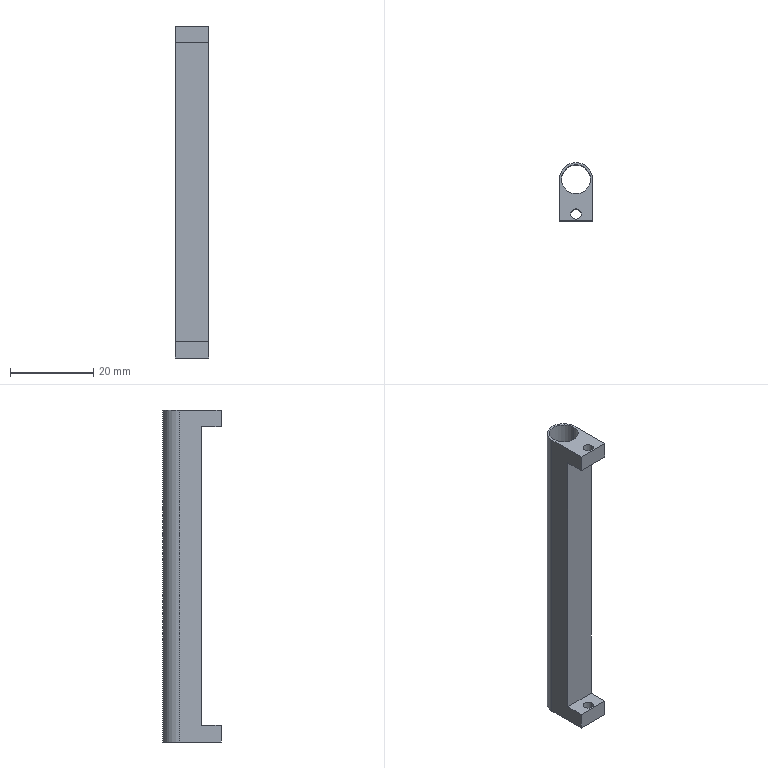Part | SolidWorks | features BaseBody 1 | 1 solid | 17 faces | box 8 x 14 x 80 mm | volume 2633 mm3 | plane 9 | cylinder 8 | commonest cylinder face diameters 2.5 x4 7 x2 8 x2
STEP:
#1=CARTESIAN_POINT('',(-1.25,-5.382,0.));
#2=VERTEX_POINT('',#1);
#3=CARTESIAN_POINT('',(1.25,-5.382,0.));
#4=VERTEX_POINT('',#3);
#5=CARTESIAN_POINT('',(0.,-5.382,0.));
#6=DIRECTION('',(0.,0.,1.));
#7=DIRECTION('',(1.,0.,0.));
#8=AXIS2_PLACEMENT_3D('',#5,#6,#7);
#9=CIRCLE('',#8,1.25);
#10=EDGE_CURVE('',#2,#4,#9,.T.);
#11=ORIENTED_EDGE('',*,*,#10,.F.);
#12=CARTESIAN_POINT('',(-1.25,-5.382,4.));
#13=VERTEX_POINT('',#12);
#14=CARTESIAN_POINT('',(-1.25,-5.382,0.));
#15=DIRECTION('',(0.,0.,1.));
#16=VECTOR('',#15,1000.);
#17=LINE('',#14,#16);
#18=EDGE_CURVE('',#2,#13,#17,.T.);
#19=ORIENTED_EDGE('',*,*,#18,.T.);
#20=CARTESIAN_POINT('',(1.25,-5.382,4.));
#21=VERTEX_POINT('',#20);
#22=CARTESIAN_POINT('',(0.,-5.382,4.));
#23=DIRECTION('',(0.,0.,1.));
#24=DIRECTION('',(1.,0.,0.));
#25=AXIS2_PLACEMENT_3D('',#22,#23,#24);
#26=CIRCLE('',#25,1.25);
#27=EDGE_CURVE('',#13,#21,#26,.T.);
#28=ORIENTED_EDGE('',*,*,#27,.T.);
#29=CARTESIAN_POINT('',(1.25,-5.382,0.));
#30=DIRECTION('',(0.,0.,1.));
#31=VECTOR('',#30,1000.);
#32=LINE('',#29,#31);
#33=EDGE_CURVE('',#4,#21,#32,.T.);
#34=ORIENTED_EDGE('',*,*,#33,.F.);
#35=EDGE_LOOP('',(#11,#19,#28,#34));
#36=FACE_OUTER_BOUND('',#35,.T.);
#37=CARTESIAN_POINT('',(0.,-5.382,0.));
#38=DIRECTION('',(0.,0.,1.));
#39=DIRECTION('',(1.,0.,0.));
#40=AXIS2_PLACEMENT_3D('',#37,#38,#39);
#41=CYLINDRICAL_SURFACE('',#40,1.25);
#42=ADVANCED_FACE('',(#36),#41,.F.);
#43=CARTESIAN_POINT('',(-1.25,-5.382,76.));
#44=VERTEX_POINT('',#43);
#45=CARTESIAN_POINT('',(1.25,-5.382,76.));
#46=VERTEX_POINT('',#45);
#47=CARTESIAN_POINT('',(0.,-5.382,76.));
#48=DIRECTION('',(0.,0.,1.));
#49=DIRECTION('',(1.,0.,0.));
#50=AXIS2_PLACEMENT_3D('',#47,#48,#49);
#51=CIRCLE('',#50,1.25);
#52=EDGE_CURVE('',#44,#46,#51,.T.);
#53=ORIENTED_EDGE('',*,*,#52,.F.);
#54=CARTESIAN_POINT('',(-1.25,-5.382,80.));
#55=VERTEX_POINT('',#54);
#56=CARTESIAN_POINT('',(-1.25,-5.382,0.));
#57=DIRECTION('',(0.,0.,1.));
#58=VECTOR('',#57,1000.);
#59=LINE('',#56,#58);
#60=EDGE_CURVE('',#44,#55,#59,.T.);
#61=ORIENTED_EDGE('',*,*,#60,.T.);
#62=CARTESIAN_POINT('',(1.25,-5.382,80.));
#63=VERTEX_POINT('',#62);
#64=CARTESIAN_POINT('',(0.,-5.382,80.));
#65=DIRECTION('',(0.,0.,1.));
#66=DIRECTION('',(1.,0.,0.));
#67=AXIS2_PLACEMENT_3D('',#64,#65,#66);
#68=CIRCLE('',#67,1.25);
#69=EDGE_CURVE('',#55,#63,#68,.T.);
#70=ORIENTED_EDGE('',*,*,#69,.T.);
#71=CARTESIAN_POINT('',(1.25,-5.382,0.));
#72=DIRECTION('',(0.,0.,1.));
#73=VECTOR('',#72,1000.);
#74=LINE('',#71,#73);
#75=EDGE_CURVE('',#46,#63,#74,.T.);
#76=ORIENTED_EDGE('',*,*,#75,.F.);
#77=EDGE_LOOP('',(#53,#61,#70,#76));
#78=FACE_OUTER_BOUND('',#77,.T.);
#79=CARTESIAN_POINT('',(0.,-5.382,0.));
#80=DIRECTION('',(0.,0.,1.));
#81=DIRECTION('',(1.,0.,0.));
#82=AXIS2_PLACEMENT_3D('',#79,#80,#81);
#83=CYLINDRICAL_SURFACE('',#82,1.25);
#84=ADVANCED_FACE('',(#78),#83,.F.);
#85=CARTESIAN_POINT('',(3.5,3.,80.));
#86=VERTEX_POINT('',#85);
#87=CARTESIAN_POINT('',(-3.5,3.,80.));
#88=VERTEX_POINT('',#87);
#89=CARTESIAN_POINT('',(0.,3.,80.));
#90=DIRECTION('',(0.,0.,-1.));
#91=DIRECTION('',(-1.,0.,0.));
#92=AXIS2_PLACEMENT_3D('',#89,#90,#91);
#93=CIRCLE('',#92,3.5);
#94=EDGE_CURVE('',#86,#88,#93,.T.);
#95=ORIENTED_EDGE('',*,*,#94,.F.);
#96=CARTESIAN_POINT('',(3.5,3.,0.));
#97=VERTEX_POINT('',#96);
#98=CARTESIAN_POINT('',(3.5,3.,80.));
#99=DIRECTION('',(0.,0.,-1.));
#100=VECTOR('',#99,1000.);
#101=LINE('',#98,#100);
#102=EDGE_CURVE('',#86,#97,#101,.T.);
#103=ORIENTED_EDGE('',*,*,#102,.T.);
#104=CARTESIAN_POINT('',(-3.5,3.,0.));
#105=VERTEX_POINT('',#104);
#106=CARTESIAN_POINT('',(0.,3.,0.));
#107=DIRECTION('',(0.,0.,-1.));
#108=DIRECTION('',(-1.,0.,0.));
#109=AXIS2_PLACEMENT_3D('',#106,#107,#108);
#110=CIRCLE('',#109,3.5);
#111=EDGE_CURVE('',#97,#105,#110,.T.);
#112=ORIENTED_EDGE('',*,*,#111,.T.);
#113=CARTESIAN_POINT('',(-3.5,3.,80.));
#114=DIRECTION('',(0.,0.,-1.));
#115=VECTOR('',#114,1000.);
#116=LINE('',#113,#115);
#117=EDGE_CURVE('',#88,#105,#116,.T.);
#118=ORIENTED_EDGE('',*,*,#117,.F.);
#119=EDGE_LOOP('',(#95,#103,#112,#118));
#120=FACE_OUTER_BOUND('',#119,.T.);
#121=CARTESIAN_POINT('',(0.,3.,80.));
#122=DIRECTION('',(0.,0.,-1.));
#123=DIRECTION('',(-1.,0.,0.));
#124=AXIS2_PLACEMENT_3D('',#121,#122,#123);
#125=CYLINDRICAL_SURFACE('',#124,3.5);
#126=ADVANCED_FACE('',(#120),#125,.F.);
#127=CARTESIAN_POINT('',(4.,-7.,4.));
#128=VERTEX_POINT('',#127);
#129=CARTESIAN_POINT('',(4.,-7.,0.));
#130=VERTEX_POINT('',#129);
#131=CARTESIAN_POINT('',(4.,-7.,80.));
#132=DIRECTION('',(0.,0.,-1.));
#133=VECTOR('',#132,1000.);
#134=LINE('',#131,#133);
#135=EDGE_CURVE('',#128,#130,#134,.T.);
#136=ORIENTED_EDGE('',*,*,#135,.F.);
#137=CARTESIAN_POINT('',(-4.,-7.,4.));
#138=VERTEX_POINT('',#137);
#139=CARTESIAN_POINT('',(-4.,-7.,4.));
#140=DIRECTION('',(1.,0.,0.));
#141=VECTOR('',#140,1000.);
#142=LINE('',#139,#141);
#143=EDGE_CURVE('',#138,#128,#142,.T.);
#144=ORIENTED_EDGE('',*,*,#143,.F.);
#145=CARTESIAN_POINT('',(-4.,-7.,0.));
#146=VERTEX_POINT('',#145);
#147=CARTESIAN_POINT('',(-4.,-7.,80.));
#148=DIRECTION('',(0.,0.,-1.));
#149=VECTOR('',#148,1000.);
#150=LINE('',#147,#149);
#151=EDGE_CURVE('',#138,#146,#150,.T.);
#152=ORIENTED_EDGE('',*,*,#151,.T.);
#153=CARTESIAN_POINT('',(-4.,-7.,0.));
#154=DIRECTION('',(1.,0.,0.));
#155=VECTOR('',#154,1000.);
#156=LINE('',#153,#155);
#157=EDGE_CURVE('',#146,#130,#156,.T.);
#158=ORIENTED_EDGE('',*,*,#157,.T.);
#159=EDGE_LOOP('',(#136,#144,#152,#158));
#160=FACE_OUTER_BOUND('',#159,.T.);
#161=CARTESIAN_POINT('',(-4.,-7.,80.));
#162=DIRECTION('',(0.,1.,0.));
#163=DIRECTION('',(0.,0.,1.));
#164=AXIS2_PLACEMENT_3D('',#161,#162,#163);
#165=PLANE('',#164);
#166=ADVANCED_FACE('',(#160),#165,.F.);
#167=CARTESIAN_POINT('',(-4.,-7.,80.));
#168=VERTEX_POINT('',#167);
#169=CARTESIAN_POINT('',(-4.,-7.,76.));
#170=VERTEX_POINT('',#169);
#171=CARTESIAN_POINT('',(-4.,-7.,80.));
#172=DIRECTION('',(0.,0.,-1.));
#173=VECTOR('',#172,1000.);
#174=LINE('',#171,#173);
#175=EDGE_CURVE('',#168,#170,#174,.T.);
#176=ORIENTED_EDGE('',*,*,#175,.T.);
#177=CARTESIAN_POINT('',(4.,-7.,76.));
#178=VERTEX_POINT('',#177);
#179=CARTESIAN_POINT('',(-4.,-7.,76.));
#180=DIRECTION('',(1.,0.,0.));
#181=VECTOR('',#180,1000.);
#182=LINE('',#179,#181);
#183=EDGE_CURVE('',#170,#178,#182,.T.);
#184=ORIENTED_EDGE('',*,*,#183,.T.);
#185=CARTESIAN_POINT('',(4.,-7.,80.));
#186=VERTEX_POINT('',#185);
#187=CARTESIAN_POINT('',(4.,-7.,80.));
#188=DIRECTION('',(0.,0.,-1.));
#189=VECTOR('',#188,1000.);
#190=LINE('',#187,#189);
#191=EDGE_CURVE('',#186,#178,#190,.T.);
#192=ORIENTED_EDGE('',*,*,#191,.F.);
#193=CARTESIAN_POINT('',(-4.,-7.,80.));
#194=DIRECTION('',(1.,0.,0.));
#195=VECTOR('',#194,1000.);
#196=LINE('',#193,#195);
#197=EDGE_CURVE('',#168,#186,#196,.T.);
#198=ORIENTED_EDGE('',*,*,#197,.F.);
#199=EDGE_LOOP('',(#176,#184,#192,#198));
#200=FACE_OUTER_BOUND('',#199,.T.);
#201=CARTESIAN_POINT('',(-4.,-7.,80.));
#202=DIRECTION('',(0.,1.,0.));
#203=DIRECTION('',(0.,0.,1.));
#204=AXIS2_PLACEMENT_3D('',#201,#202,#203);
#205=PLANE('',#204);
#206=ADVANCED_FACE('',(#200),#205,.F.);
#207=CARTESIAN_POINT('',(4.,-2.382,4.));
#208=VERTEX_POINT('',#207);
#209=CARTESIAN_POINT('',(4.,-2.382,76.));
#210=VERTEX_POINT('',#209);
#211=CARTESIAN_POINT('',(4.,-2.382,4.));
#212=DIRECTION('',(0.,0.,1.));
#213=VECTOR('',#212,1000.);
#214=LINE('',#211,#213);
#215=EDGE_CURVE('',#208,#210,#214,.T.);
#216=ORIENTED_EDGE('',*,*,#215,.F.);
#217=CARTESIAN_POINT('',(4.,-7.,4.));
#218=DIRECTION('',(0.,1.,0.));
#219=VECTOR('',#218,1000.);
#220=LINE('',#217,#219);
#221=EDGE_CURVE('',#128,#208,#220,.T.);
#222=ORIENTED_EDGE('',*,*,#221,.F.);
#223=ORIENTED_EDGE('',*,*,#135,.T.);
#224=CARTESIAN_POINT('',(4.,3.,0.));
#225=VERTEX_POINT('',#224);
#226=CARTESIAN_POINT('',(4.,7.,0.));
#227=DIRECTION('',(0.,1.,0.));
#228=VECTOR('',#227,1000.);
#229=LINE('',#226,#228);
#230=EDGE_CURVE('',#130,#225,#229,.T.);
#231=ORIENTED_EDGE('',*,*,#230,.T.);
#232=CARTESIAN_POINT('',(4.,3.,80.));
#233=VERTEX_POINT('',#232);
#234=CARTESIAN_POINT('',(4.,3.,80.));
#235=DIRECTION('',(0.,0.,1.));
#236=VECTOR('',#235,1000.);
#237=LINE('',#234,#236);
#238=EDGE_CURVE('',#225,#233,#237,.T.);
#239=ORIENTED_EDGE('',*,*,#238,.T.);
#240=CARTESIAN_POINT('',(4.,7.,80.));
#241=DIRECTION('',(0.,1.,0.));
#242=VECTOR('',#241,1000.);
#243=LINE('',#240,#242);
#244=EDGE_CURVE('',#186,#233,#243,.T.);
#245=ORIENTED_EDGE('',*,*,#244,.F.);
#246=ORIENTED_EDGE('',*,*,#191,.T.);
#247=CARTESIAN_POINT('',(4.,-7.,76.));
#248=DIRECTION('',(0.,-1.,0.));
#249=VECTOR('',#248,1000.);
#250=LINE('',#247,#249);
#251=EDGE_CURVE('',#210,#178,#250,.T.);
#252=ORIENTED_EDGE('',*,*,#251,.F.);
#253=EDGE_LOOP('',(#216,#222,#223,#231,#239,#245,#246,#252));
#254=FACE_OUTER_BOUND('',#253,.T.);
#255=CARTESIAN_POINT('',(4.,7.,80.));
#256=DIRECTION('',(-1.,0.,0.));
#257=DIRECTION('',(0.,0.,1.));
#258=AXIS2_PLACEMENT_3D('',#255,#256,#257);
#259=PLANE('',#258);
#260=ADVANCED_FACE('',(#254),#259,.F.);
#261=ORIENTED_EDGE('',*,*,#151,.F.);
#262=CARTESIAN_POINT('',(-4.,-2.382,4.));
#263=VERTEX_POINT('',#262);
#264=CARTESIAN_POINT('',(-4.,7.,4.));
#265=DIRECTION('',(0.,1.,0.));
#266=VECTOR('',#265,1000.);
#267=LINE('',#264,#266);
#268=EDGE_CURVE('',#138,#263,#267,.T.);
#269=ORIENTED_EDGE('',*,*,#268,.T.);
#270=CARTESIAN_POINT('',(-4.,-2.382,76.));
#271=VERTEX_POINT('',#270);
#272=CARTESIAN_POINT('',(-4.,-2.382,80.));
#273=DIRECTION('',(0.,0.,1.));
#274=VECTOR('',#273,1000.);
#275=LINE('',#272,#274);
#276=EDGE_CURVE('',#263,#271,#275,.T.);
#277=ORIENTED_EDGE('',*,*,#276,.T.);
#278=CARTESIAN_POINT('',(-4.,7.,76.));
#279=DIRECTION('',(0.,-1.,0.));
#280=VECTOR('',#279,1000.);
#281=LINE('',#278,#280);
#282=EDGE_CURVE('',#271,#170,#281,.T.);
#283=ORIENTED_EDGE('',*,*,#282,.T.);
#284=ORIENTED_EDGE('',*,*,#175,.F.);
#285=CARTESIAN_POINT('',(-4.,3.,80.));
#286=VERTEX_POINT('',#285);
#287=CARTESIAN_POINT('',(-4.,7.,80.));
#288=DIRECTION('',(0.,-1.,0.));
#289=VECTOR('',#288,1000.);
#290=LINE('',#287,#289);
#291=EDGE_CURVE('',#286,#168,#290,.T.);
#292=ORIENTED_EDGE('',*,*,#291,.F.);
#293=CARTESIAN_POINT('',(-4.,3.,0.));
#294=VERTEX_POINT('',#293);
#295=CARTESIAN_POINT('',(-4.,3.,80.));
#296=DIRECTION('',(0.,0.,-1.));
#297=VECTOR('',#296,1000.);
#298=LINE('',#295,#297);
#299=EDGE_CURVE('',#286,#294,#298,.T.);
#300=ORIENTED_EDGE('',*,*,#299,.T.);
#301=CARTESIAN_POINT('',(-4.,7.,0.));
#302=DIRECTION('',(0.,-1.,0.));
#303=VECTOR('',#302,1000.);
#304=LINE('',#301,#303);
#305=EDGE_CURVE('',#294,#146,#304,.T.);
#306=ORIENTED_EDGE('',*,*,#305,.T.);
#307=EDGE_LOOP('',(#261,#269,#277,#283,#284,#292,#300,#306));
#308=FACE_OUTER_BOUND('',#307,.T.);
#309=CARTESIAN_POINT('',(-4.,7.,80.));
#310=DIRECTION('',(1.,0.,0.));
#311=DIRECTION('',(0.,0.,-1.));
#312=AXIS2_PLACEMENT_3D('',#309,#310,#311);
#313=PLANE('',#312);
#314=ADVANCED_FACE('',(#308),#313,.F.);
#315=CARTESIAN_POINT('',(0.,-5.382,80.));
#316=DIRECTION('',(0.,0.,1.));
#317=DIRECTION('',(1.,0.,0.));
#318=AXIS2_PLACEMENT_3D('',#315,#316,#317);
#319=CIRCLE('',#318,1.25);
#320=EDGE_CURVE('',#63,#55,#319,.T.);
#321=ORIENTED_EDGE('',*,*,#320,.F.);
#322=ORIENTED_EDGE('',*,*,#69,.F.);
#323=EDGE_LOOP('',(#321,#322));
#324=FACE_BOUND('',#323,.T.);
#325=CARTESIAN_POINT('',(0.,3.,80.));
#326=DIRECTION('',(0.,0.,-1.));
#327=DIRECTION('',(-1.,0.,0.));
#328=AXIS2_PLACEMENT_3D('',#325,#326,#327);
#329=CIRCLE('',#328,3.5);
#330=EDGE_CURVE('',#88,#86,#329,.T.);
#331=ORIENTED_EDGE('',*,*,#330,.T.);
#332=ORIENTED_EDGE('',*,*,#94,.T.);
#333=EDGE_LOOP('',(#331,#332));
#334=FACE_BOUND('',#333,.T.);
#335=ORIENTED_EDGE('',*,*,#244,.T.);
#336=CARTESIAN_POINT('',(0.,7.,80.));
#337=VERTEX_POINT('',#336);
#338=CARTESIAN_POINT('',(0.,3.,80.));
#339=DIRECTION('',(0.,0.,1.));
#340=DIRECTION('',(1.,0.,0.));
#341=AXIS2_PLACEMENT_3D('',#338,#339,#340);
#342=CIRCLE('',#341,4.);
#343=EDGE_CURVE('',#233,#337,#342,.T.);
#344=ORIENTED_EDGE('',*,*,#343,.T.);
#345=CARTESIAN_POINT('',(0.,3.,80.));
#346=DIRECTION('',(0.,0.,1.));
#347=DIRECTION('',(1.,0.,0.));
#348=AXIS2_PLACEMENT_3D('',#345,#346,#347);
#349=CIRCLE('',#348,4.);
#350=EDGE_CURVE('',#337,#286,#349,.T.);
#351=ORIENTED_EDGE('',*,*,#350,.T.);
#352=ORIENTED_EDGE('',*,*,#291,.T.);
#353=ORIENTED_EDGE('',*,*,#197,.T.);
#354=EDGE_LOOP('',(#335,#344,#351,#352,#353));
#355=FACE_OUTER_BOUND('',#354,.T.);
#356=CARTESIAN_POINT('',(0.,0.,80.));
#357=DIRECTION('',(0.,0.,1.));
#358=DIRECTION('',(1.,0.,0.));
#359=AXIS2_PLACEMENT_3D('',#356,#357,#358);
#360=PLANE('',#359);
#361=ADVANCED_FACE('',(#324,#334,#355),#360,.T.);
#362=CARTESIAN_POINT('',(0.,-5.382,0.));
#363=DIRECTION('',(0.,0.,1.));
#364=DIRECTION('',(1.,0.,0.));
#365=AXIS2_PLACEMENT_3D('',#362,#363,#364);
#366=CIRCLE('',#365,1.25);
#367=EDGE_CURVE('',#4,#2,#366,.T.);
#368=ORIENTED_EDGE('',*,*,#367,.T.);
#369=ORIENTED_EDGE('',*,*,#10,.T.);
#370=EDGE_LOOP('',(#368,#369));
#371=FACE_BOUND('',#370,.T.);
#372=CARTESIAN_POINT('',(0.,3.,0.));
#373=DIRECTION('',(0.,0.,-1.));
#374=DIRECTION('',(-1.,0.,0.));
#375=AXIS2_PLACEMENT_3D('',#372,#373,#374);
#376=CIRCLE('',#375,3.5);
#377=EDGE_CURVE('',#105,#97,#376,.T.);
#378=ORIENTED_EDGE('',*,*,#377,.F.);
#379=ORIENTED_EDGE('',*,*,#111,.F.);
#380=EDGE_LOOP('',(#378,#379));
#381=FACE_BOUND('',#380,.T.);
#382=CARTESIAN_POINT('',(0.,7.,0.));
#383=VERTEX_POINT('',#382);
#384=CARTESIAN_POINT('',(0.,3.,0.));
#385=DIRECTION('',(0.,0.,-1.));
#386=DIRECTION('',(1.,0.,0.));
#387=AXIS2_PLACEMENT_3D('',#384,#385,#386);
#388=CIRCLE('',#387,4.);
#389=EDGE_CURVE('',#294,#383,#388,.T.);
#390=ORIENTED_EDGE('',*,*,#389,.T.);
#391=CARTESIAN_POINT('',(0.,3.,0.));
#392=DIRECTION('',(0.,0.,-1.));
#393=DIRECTION('',(1.,0.,0.));
#394=AXIS2_PLACEMENT_3D('',#391,#392,#393);
#395=CIRCLE('',#394,4.);
#396=EDGE_CURVE('',#383,#225,#395,.T.);
#397=ORIENTED_EDGE('',*,*,#396,.T.);
#398=ORIENTED_EDGE('',*,*,#230,.F.);
#399=ORIENTED_EDGE('',*,*,#157,.F.);
#400=ORIENTED_EDGE('',*,*,#305,.F.);
#401=EDGE_LOOP('',(#390,#397,#398,#399,#400));
#402=FACE_OUTER_BOUND('',#401,.T.);
#403=CARTESIAN_POINT('',(0.,0.,0.));
#404=DIRECTION('',(0.,0.,1.));
#405=DIRECTION('',(1.,0.,0.));
#406=AXIS2_PLACEMENT_3D('',#403,#404,#405);
#407=PLANE('',#406);
#408=ADVANCED_FACE('',(#371,#381,#402),#407,.F.);
#409=ORIENTED_EDGE('',*,*,#299,.F.);
#410=ORIENTED_EDGE('',*,*,#350,.F.);
#411=CARTESIAN_POINT('',(0.,7.,80.));
#412=DIRECTION('',(0.,0.,1.));
#413=VECTOR('',#412,1000.);
#414=LINE('',#411,#413);
#415=EDGE_CURVE('',#383,#337,#414,.T.);
#416=ORIENTED_EDGE('',*,*,#415,.F.);
#417=ORIENTED_EDGE('',*,*,#389,.F.);
#418=EDGE_LOOP('',(#409,#410,#416,#417));
#419=FACE_OUTER_BOUND('',#418,.T.);
#420=CARTESIAN_POINT('',(0.,3.,80.));
#421=DIRECTION('',(0.,0.,-1.));
#422=DIRECTION('',(-1.,0.,0.));
#423=AXIS2_PLACEMENT_3D('',#420,#421,#422);
#424=CYLINDRICAL_SURFACE('',#423,4.);
#425=ADVANCED_FACE('',(#419),#424,.T.);
#426=ORIENTED_EDGE('',*,*,#343,.F.);
#427=ORIENTED_EDGE('',*,*,#238,.F.);
#428=ORIENTED_EDGE('',*,*,#396,.F.);
#429=ORIENTED_EDGE('',*,*,#415,.T.);
#430=EDGE_LOOP('',(#426,#427,#428,#429));
#431=FACE_OUTER_BOUND('',#430,.T.);
#432=CARTESIAN_POINT('',(0.,3.,80.));
#433=DIRECTION('',(0.,0.,-1.));
#434=DIRECTION('',(-1.,0.,0.));
#435=AXIS2_PLACEMENT_3D('',#432,#433,#434);
#436=CYLINDRICAL_SURFACE('',#435,4.);
#437=ADVANCED_FACE('',(#431),#436,.T.);
#438=ORIENTED_EDGE('',*,*,#102,.F.);
#439=ORIENTED_EDGE('',*,*,#330,.F.);
#440=ORIENTED_EDGE('',*,*,#117,.T.);
#441=ORIENTED_EDGE('',*,*,#377,.T.);
#442=EDGE_LOOP('',(#438,#439,#440,#441));
#443=FACE_OUTER_BOUND('',#442,.T.);
#444=CARTESIAN_POINT('',(0.,3.,80.));
#445=DIRECTION('',(0.,0.,-1.));
#446=DIRECTION('',(-1.,0.,0.));
#447=AXIS2_PLACEMENT_3D('',#444,#445,#446);
#448=CYLINDRICAL_SURFACE('',#447,3.5);
#449=ADVANCED_FACE('',(#443),#448,.F.);
#450=CARTESIAN_POINT('',(0.,-5.382,4.));
#451=DIRECTION('',(0.,0.,1.));
#452=DIRECTION('',(1.,0.,0.));
#453=AXIS2_PLACEMENT_3D('',#450,#451,#452);
#454=CIRCLE('',#453,1.25);
#455=EDGE_CURVE('',#21,#13,#454,.T.);
#456=ORIENTED_EDGE('',*,*,#455,.F.);
#457=ORIENTED_EDGE('',*,*,#27,.F.);
#458=EDGE_LOOP('',(#456,#457));
#459=FACE_BOUND('',#458,.T.);
#460=ORIENTED_EDGE('',*,*,#143,.T.);
#461=ORIENTED_EDGE('',*,*,#221,.T.);
#462=CARTESIAN_POINT('',(-76.,-2.382,4.));
#463=DIRECTION('',(1.,0.,0.));
#464=VECTOR('',#463,1000.);
#465=LINE('',#462,#464);
#466=EDGE_CURVE('',#263,#208,#465,.T.);
#467=ORIENTED_EDGE('',*,*,#466,.F.);
#468=ORIENTED_EDGE('',*,*,#268,.F.);
#469=EDGE_LOOP('',(#460,#461,#467,#468));
#470=FACE_OUTER_BOUND('',#469,.T.);
#471=CARTESIAN_POINT('',(0.,-5.382,4.));
#472=DIRECTION('',(0.,0.,1.));
#473=DIRECTION('',(1.,0.,0.));
#474=AXIS2_PLACEMENT_3D('',#471,#472,#473);
#475=PLANE('',#474);
#476=ADVANCED_FACE('',(#459,#470),#475,.T.);
#477=CARTESIAN_POINT('',(0.,-5.382,76.));
#478=DIRECTION('',(0.,0.,1.));
#479=DIRECTION('',(1.,0.,0.));
#480=AXIS2_PLACEMENT_3D('',#477,#478,#479);
#481=CIRCLE('',#480,1.25);
#482=EDGE_CURVE('',#46,#44,#481,.T.);
#483=ORIENTED_EDGE('',*,*,#482,.T.);
#484=ORIENTED_EDGE('',*,*,#52,.T.);
#485=EDGE_LOOP('',(#483,#484));
#486=FACE_BOUND('',#485,.T.);
#487=ORIENTED_EDGE('',*,*,#183,.F.);
#488=ORIENTED_EDGE('',*,*,#282,.F.);
#489=CARTESIAN_POINT('',(-76.,-2.382,76.));
#490=DIRECTION('',(1.,0.,0.));
#491=VECTOR('',#490,1000.);
#492=LINE('',#489,#491);
#493=EDGE_CURVE('',#271,#210,#492,.T.);
#494=ORIENTED_EDGE('',*,*,#493,.T.);
#495=ORIENTED_EDGE('',*,*,#251,.T.);
#496=EDGE_LOOP('',(#487,#488,#494,#495));
#497=FACE_OUTER_BOUND('',#496,.T.);
#498=CARTESIAN_POINT('',(0.,-5.382,76.));
#499=DIRECTION('',(0.,0.,1.));
#500=DIRECTION('',(1.,0.,0.));
#501=AXIS2_PLACEMENT_3D('',#498,#499,#500);
#502=PLANE('',#501);
#503=ADVANCED_FACE('',(#486,#497),#502,.F.);
#504=ORIENTED_EDGE('',*,*,#60,.F.);
#505=ORIENTED_EDGE('',*,*,#482,.F.);
#506=ORIENTED_EDGE('',*,*,#75,.T.);
#507=ORIENTED_EDGE('',*,*,#320,.T.);
#508=EDGE_LOOP('',(#504,#505,#506,#507));
#509=FACE_OUTER_BOUND('',#508,.T.);
#510=CARTESIAN_POINT('',(0.,-5.382,0.));
#511=DIRECTION('',(0.,0.,1.));
#512=DIRECTION('',(1.,0.,0.));
#513=AXIS2_PLACEMENT_3D('',#510,#511,#512);
#514=CYLINDRICAL_SURFACE('',#513,1.25);
#515=ADVANCED_FACE('',(#509),#514,.F.);
#516=ORIENTED_EDGE('',*,*,#18,.F.);
#517=ORIENTED_EDGE('',*,*,#367,.F.);
#518=ORIENTED_EDGE('',*,*,#33,.T.);
#519=ORIENTED_EDGE('',*,*,#455,.T.);
#520=EDGE_LOOP('',(#516,#517,#518,#519));
#521=FACE_OUTER_BOUND('',#520,.T.);
#522=CARTESIAN_POINT('',(0.,-5.382,0.));
#523=DIRECTION('',(0.,0.,1.));
#524=DIRECTION('',(1.,0.,0.));
#525=AXIS2_PLACEMENT_3D('',#522,#523,#524);
#526=CYLINDRICAL_SURFACE('',#525,1.25);
#527=ADVANCED_FACE('',(#521),#526,.F.);
#528=ORIENTED_EDGE('',*,*,#466,.T.);
#529=ORIENTED_EDGE('',*,*,#215,.T.);
#530=ORIENTED_EDGE('',*,*,#493,.F.);
#531=ORIENTED_EDGE('',*,*,#276,.F.);
#532=EDGE_LOOP('',(#528,#529,#530,#531));
#533=FACE_OUTER_BOUND('',#532,.T.);
#534=CARTESIAN_POINT('',(-76.,-2.382,4.));
#535=DIRECTION('',(0.,1.,0.));
#536=DIRECTION('',(0.,0.,1.));
#537=AXIS2_PLACEMENT_3D('',#534,#535,#536);
#538=PLANE('',#537);
#539=ADVANCED_FACE('',(#533),#538,.F.);
#540=CLOSED_SHELL('',(#42,#84,#126,#166,#206,#260,#314,#361,#408,#425,#437,#449,#476,#503,#515,#527,#539));
#541=MANIFOLD_SOLID_BREP('',#540);
#542=CARTESIAN_POINT('',(0.,0.,0.));
#543=DIRECTION('',(0.,0.,1.));
#544=DIRECTION('',(1.,0.,0.));
#545=AXIS2_PLACEMENT_3D('',#542,#543,#544);
#546=(LENGTH_UNIT()NAMED_UNIT(*)SI_UNIT(.MILLI.,.METRE.));
#547=UNCERTAINTY_MEASURE_WITH_UNIT(LENGTH_MEASURE(0.00001),#546,'','');
#548=(NAMED_UNIT(*)PLANE_ANGLE_UNIT()SI_UNIT($,.RADIAN.));
#549=(NAMED_UNIT(*)SI_UNIT($,.STERADIAN.)SOLID_ANGLE_UNIT());
#550=(GEOMETRIC_REPRESENTATION_CONTEXT(3)GLOBAL_UNCERTAINTY_ASSIGNED_CONTEXT((#547))GLOBAL_UNIT_ASSIGNED_CONTEXT((#546,#548,#549))REPRESENTATION_CONTEXT('',''));
#551=ADVANCED_BREP_SHAPE_REPRESENTATION('',(#541,#545),#550);